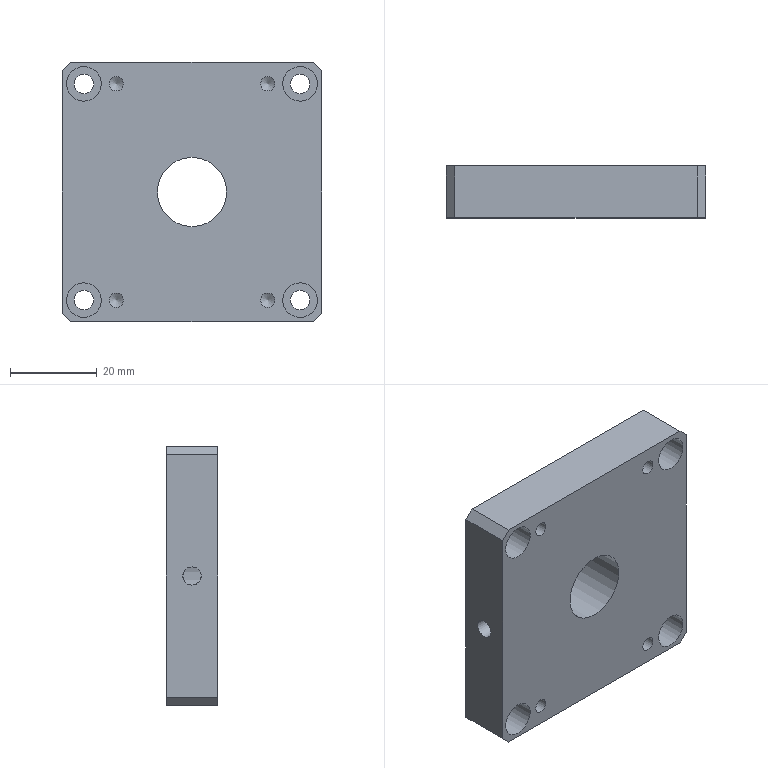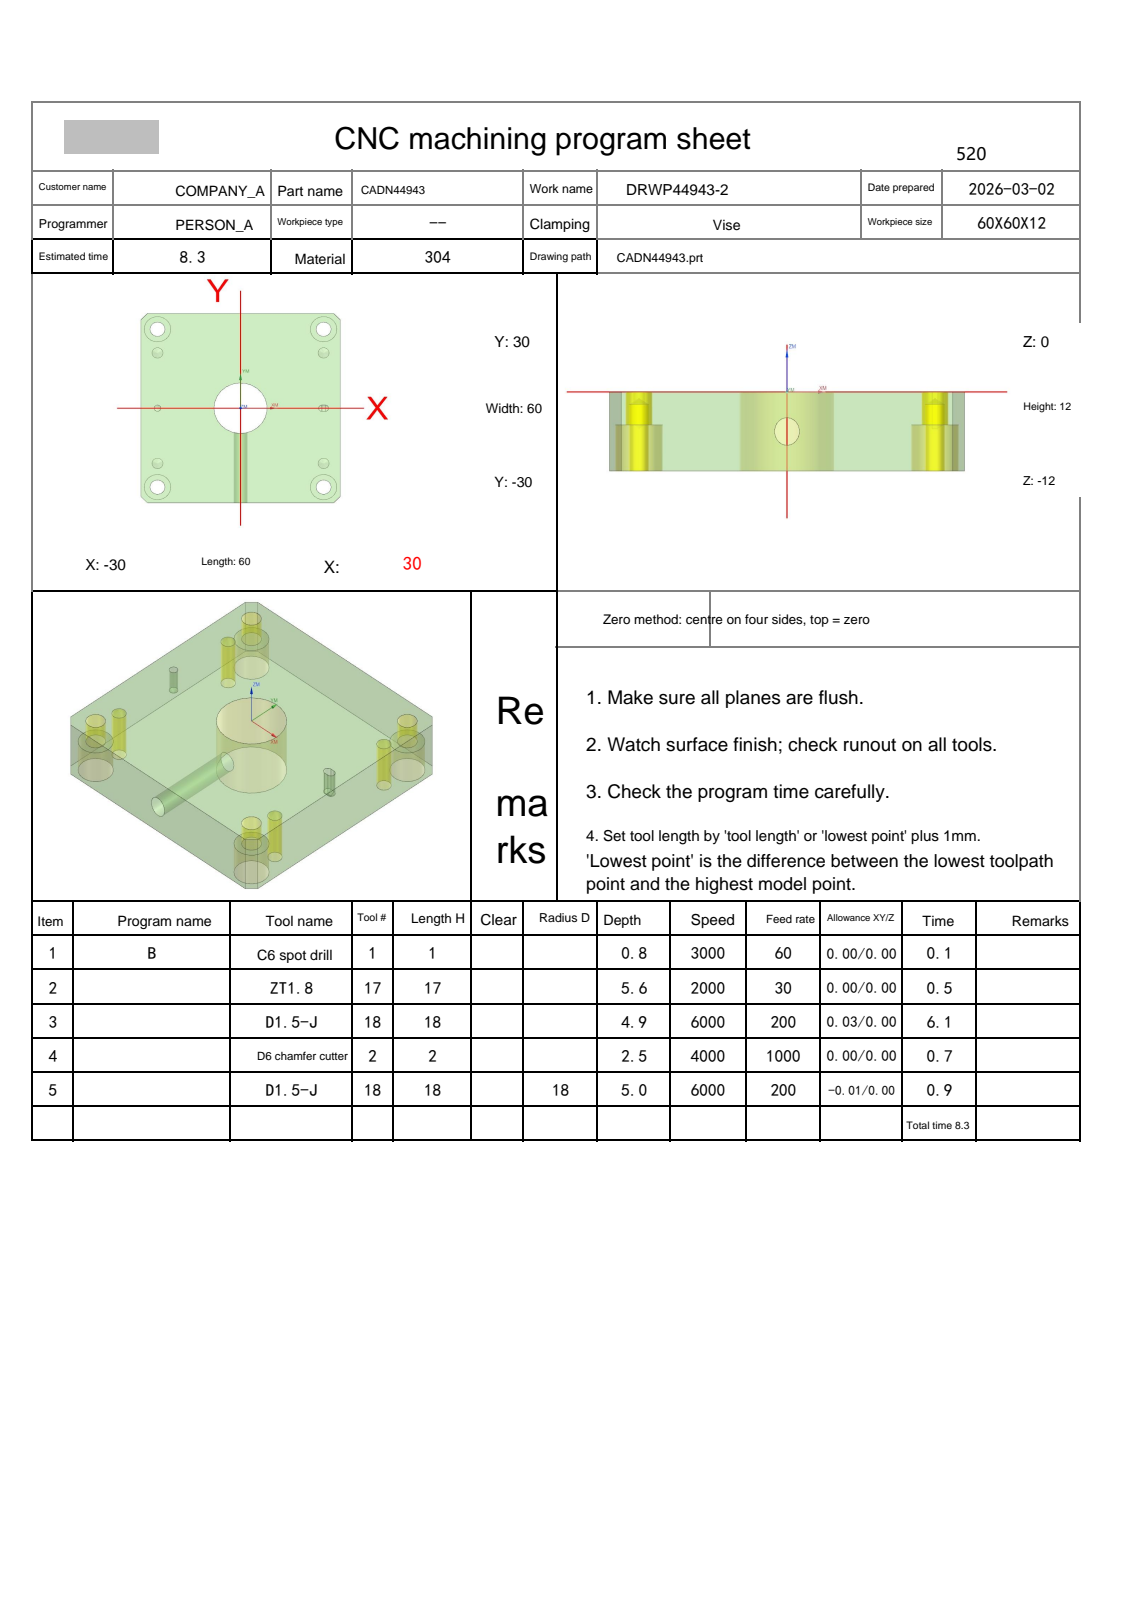NC program | NX | posted by the shop | part box 60 x 12 x 60 mm
Lines 1 to 41 of 3254:
%
O0001
(Machine time: 9.17 MIN)
(===Total Tool:4===)
(T1=C6 spot drill   D=6.   R=0.   D-  H01 Z=-0.8  )
(T17=ZT1.8  D=1.6  DR_a=118 D-  H17 Z=-5.6  )
(T18=D1.5-J D=1.5  R=0.   D-  H18 Z=-5.   )
(T2=D6 chamfer cutter   D=6.   R=0.   D-  H02 Z=-2.55 )
G80 G90 G17 G49 G40
G91 G28 Z0
M01
N1 T01 M06
(C6 spot drill  D=6. R=0. H=01 ce=0.00 di=0.00)
G00 G90 G54 X-25. Y0.0 M03 S3000
G43 H01 Z50.
M08
G98 G81 X-25. Y0.0 Z-.8 R1. F60.
X24.5
G80
G00 Z50.
G91 G28 Z0.0
M05
M09
G91 G28 Z0.0
M01
N2 T17 M06
(ZT1.8 D=1.6 DR_a=118 H=17)
G00 G90 G54 X-25. Y0.0 M03 S2000
G43 H17 Z50.
M08
G98 G83 X-25. Y0.0 Z-5.601 R1. F30. Q1.
X24.5
G80
G00 Z50.
G91 G28 Z0.0
M05
M09
G91 G28 Z0.0
M01